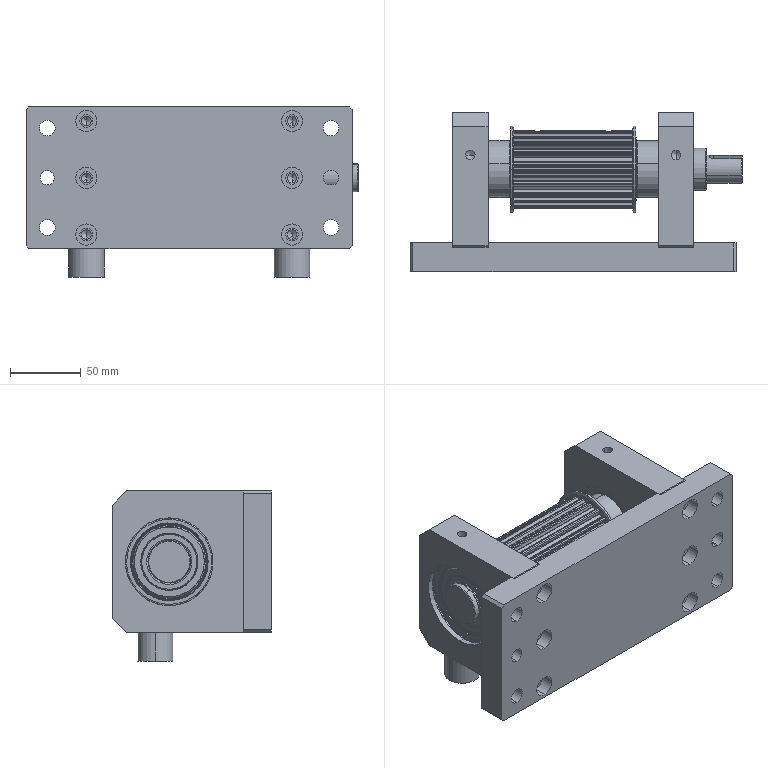Part | SolidWorks | 13 solids | 786 faces | box 234 x 112 x 120 mm | volume 1078897 mm3 | cylinder 423 | cone 137 | plane 122 | spline 104 | commonest cylinder face diameters 0.8 x60 1.5 x60 10.6 x54 48.99 x29 54.65 x24 6.8 x20